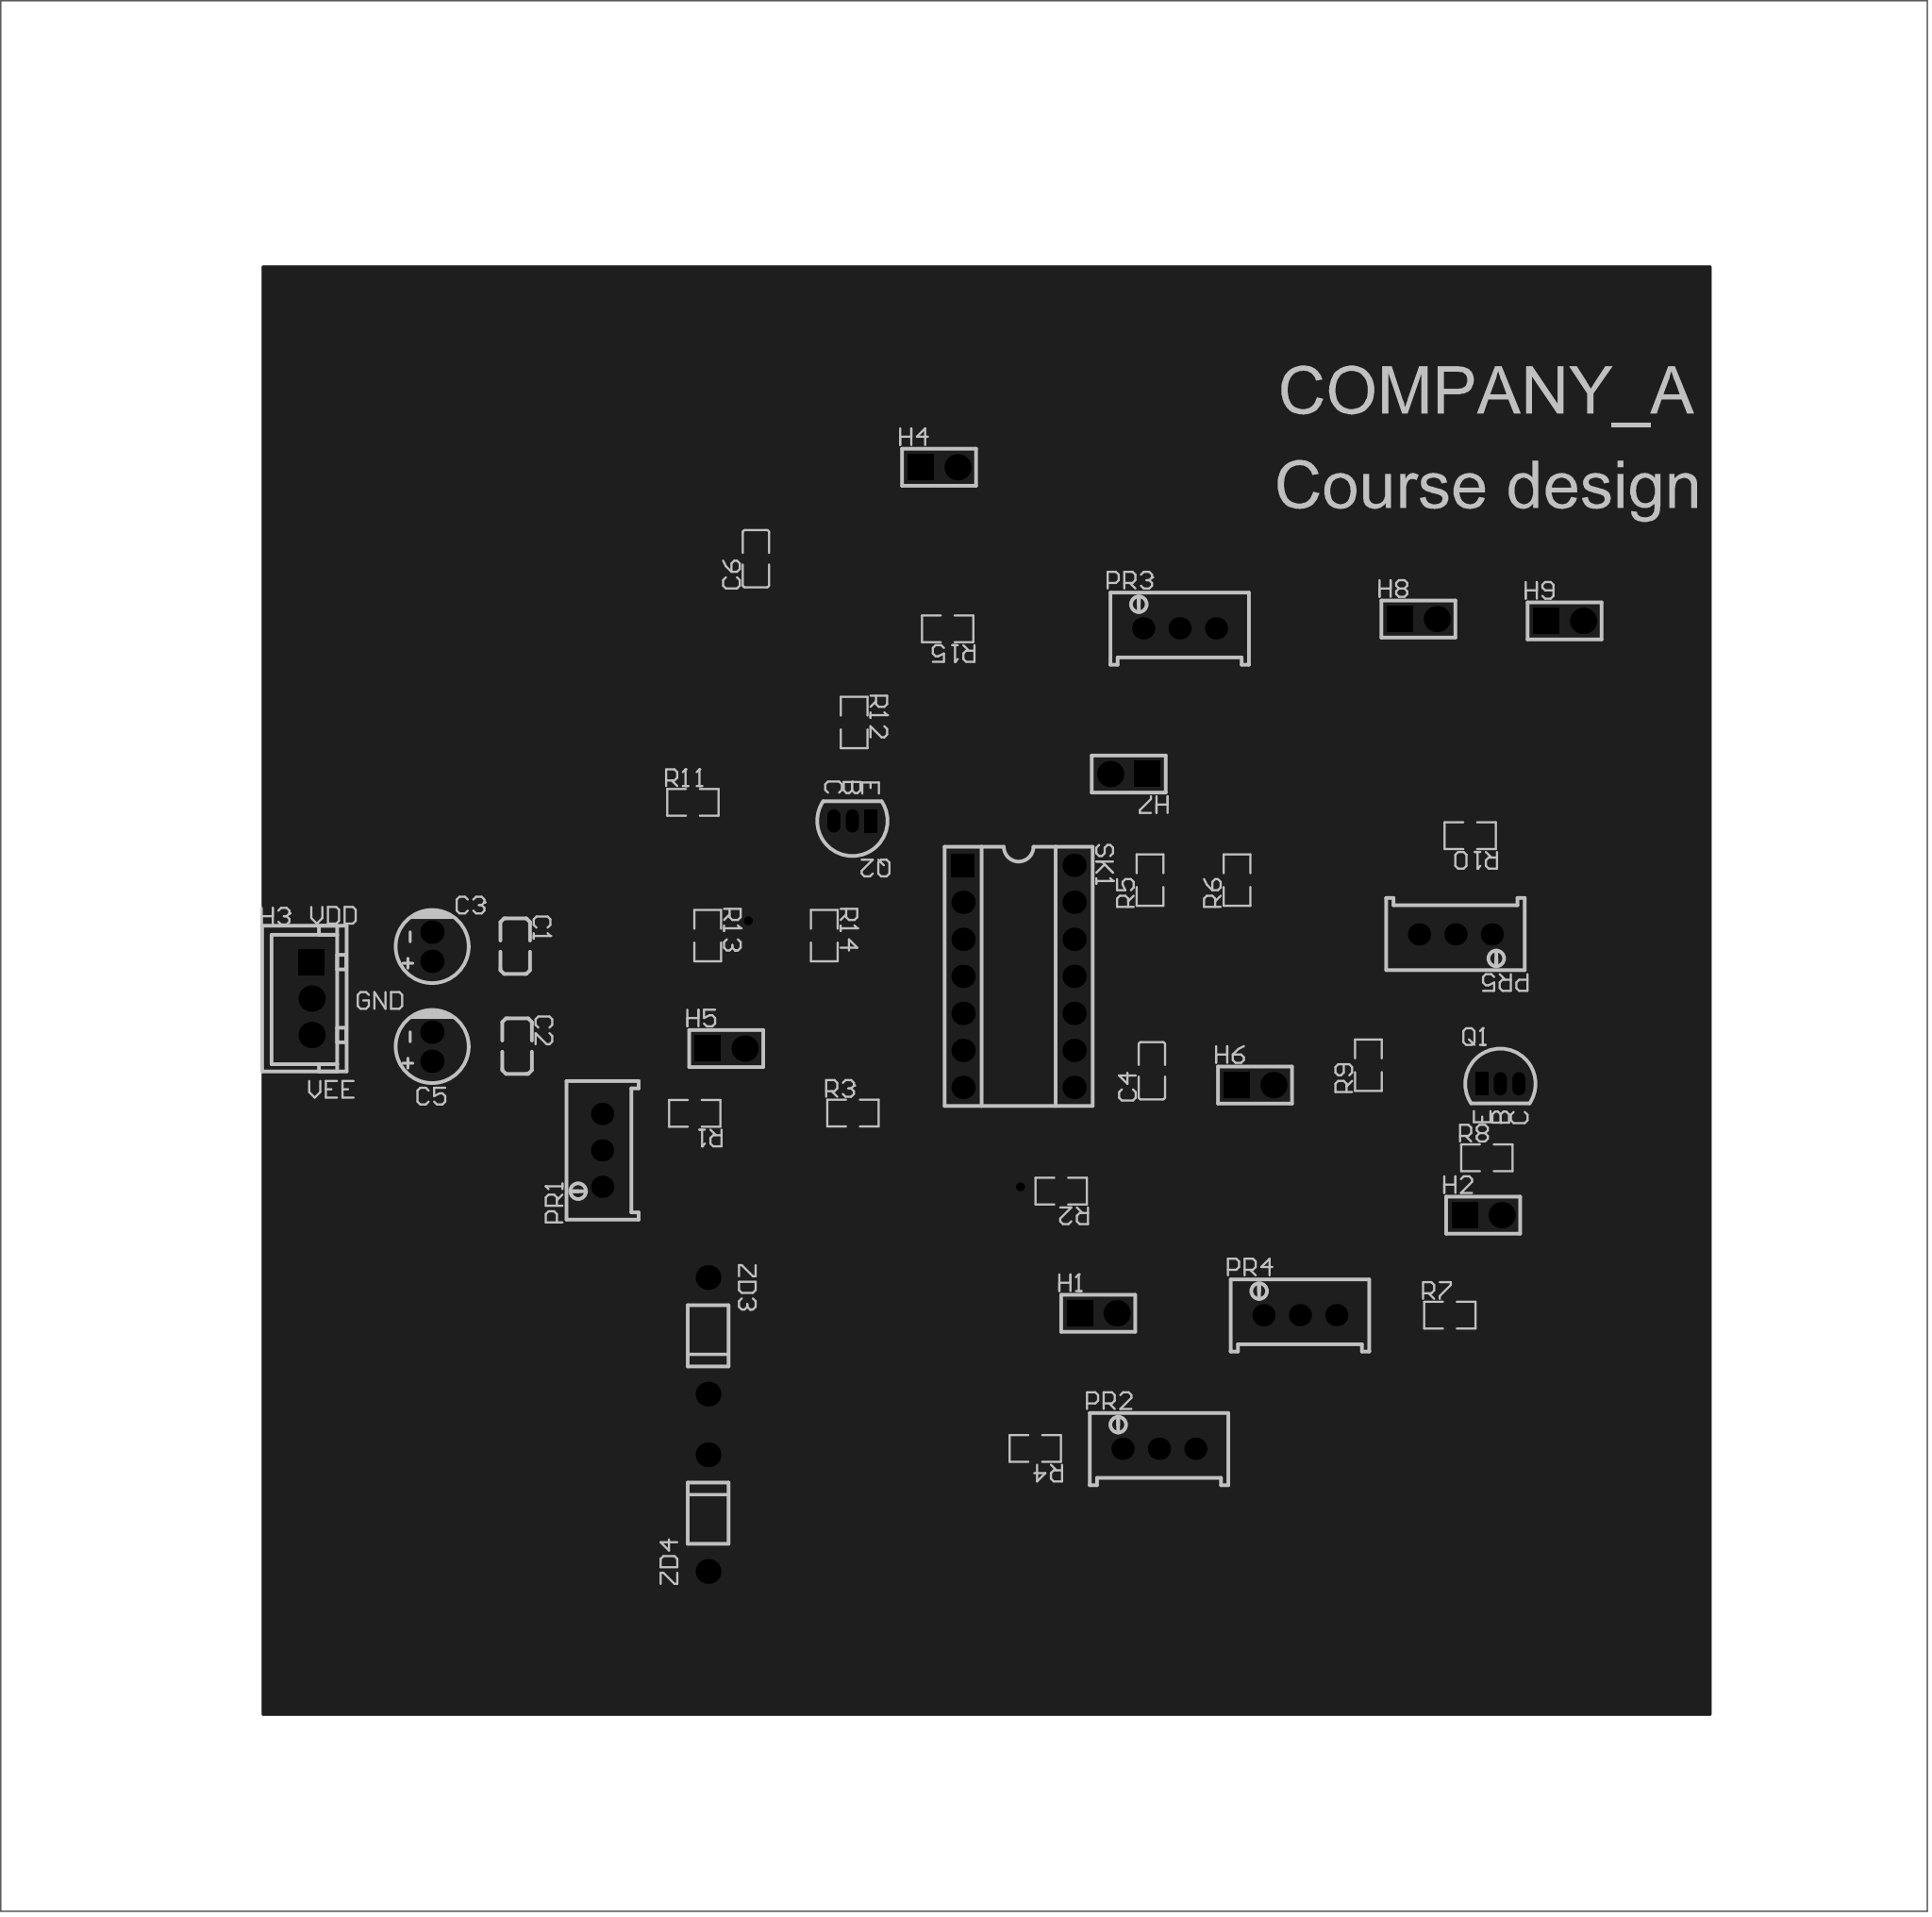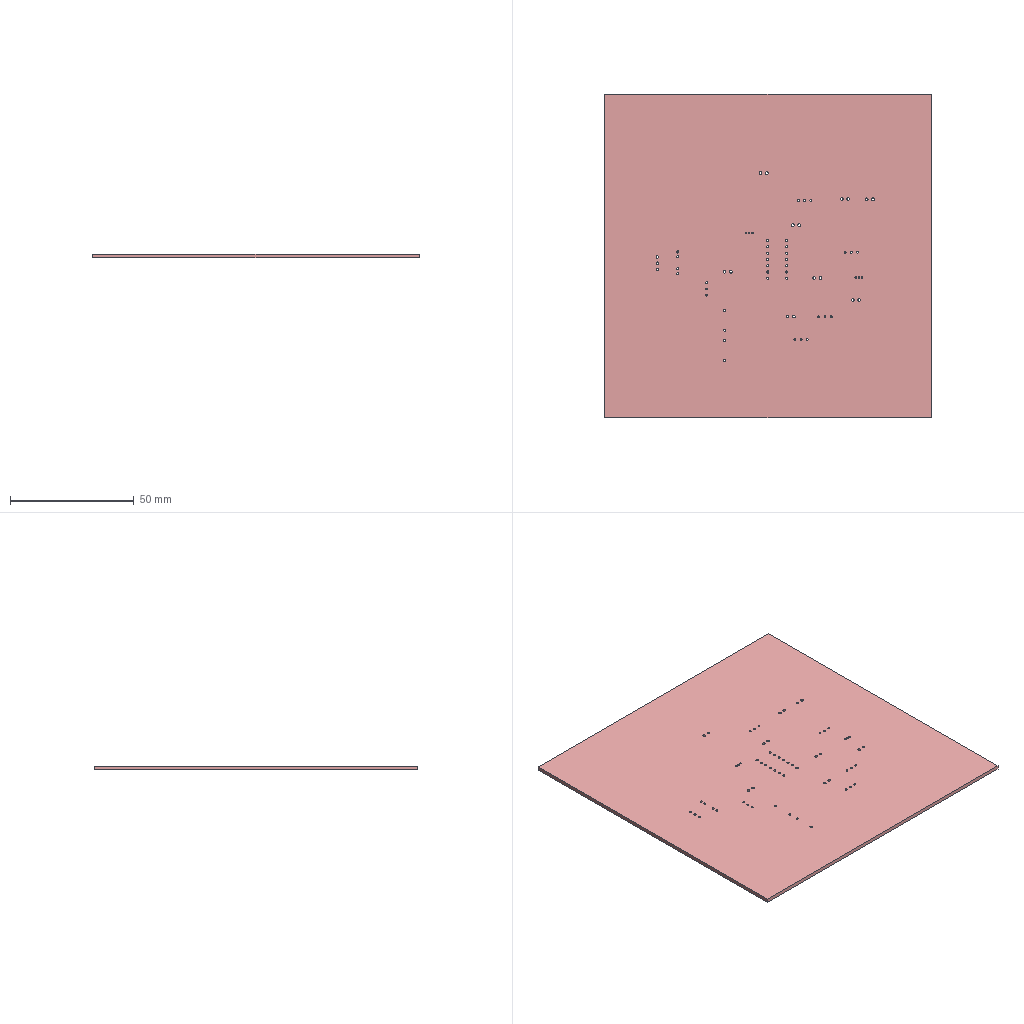Circuit board layout | Altium Designer | box 132.2 x 131.1 x 1.6 mm
Layer stack:
# Altium Designer layer stack of  (unit mm; dielectric type: 0 none, 1 core, 2 prepreg, 3 surface material)
index,name,kind,layer,copper_thickness_mm,dielectric_type,dielectric_thickness_mm,dielectric_material,dielectric_constant
0,Top Paste Mask Layer,other,,,,,,
1,Top Silkscreen Layer,other,,,,,,
2,Top Solder Mask Layer,dielectric,,,3,0.01,,3.3
3,Top Layer,copper,Top Layer,0.035,,,,
4,Dielectric1,dielectric,,,3,1.51,FR4,4.5
5,Bottom Layer,copper,Bottom Layer,0.035,,,,
6,Bottom Solder Mask Layer,dielectric,,,3,0.01,,3.3
7,Bottom Silkscreen Layer,other,,,,,,
8,Bottom Paste Mask Layer,other,,,,,,
# drill layer pairs: low layer,high layer
drill_pair,Top Layer,Bottom Layer
Part placement:
Designator,Comment,Layer,Footprint,Center-X(mm),Center-Y(mm),Rotation
C1,100nF,TopLayer,L0805,105.156,136.017,270
C2,100nF,TopLayer,L0805,105.283,129.159,270
C3,10uF,TopLayer,CAP-TH_BD5.0-P2.00-D0.5-FD-A,99.441,136.017,90
C4,22nF,TopLayer,C0805,148.844,127.508,90
C5,10uF,TopLayer,CAP-TH_BD5.0-P2.00-D0.5-FD-A,99.441,129.159,90
C6,100pF,TopLayer,C0805,121.671,162.635,90
H1,,TopLayer,HDR-TH_2P-P2.54-V-M-1,145.161,110.871,0
H2,,TopLayer,HDR-TH_2P-P2.54-V-M-1,171.577,117.602,0
H3,,TopLayer,CONN-TH_3P-P2.50_HX-XH2.54-3PZZ-B,91.186,132.461,90
H4,,TopLayer,HDR-TH_2P-P2.54-V-M-1,134.239,168.91,0
H5,,TopLayer,HDR-TH_2P-P2.54-V-M-1,119.634,129.032,0
H6,,TopLayer,HDR-TH_2P-P2.54-V-M-1,155.92,126.528,0
H7,,TopLayer,HDR-TH_2P-P2.54-V-M-1,147.256,147.864,180
H8,,TopLayer,HDR-TH_2P-P2.54-V-M-1,167.132,158.496,0
H9,,TopLayer,HDR-TH_2P-P2.54-V-M-1,177.165,158.369,0
PR1,5kΩ,TopLayer,R_3296,111.125,122.047,90
PR2,100kΩ,TopLayer,R_3296,149.333,101.578,0
PR3,10kΩ,TopLayer,R_3296,150.749,157.861,0
PR4,10kΩ,TopLayer,R_3296,159.004,110.744,0
PR5,10kΩ,TopLayer,R_3296,169.677,136.865,180
Q1,,TopLayer,S8050_TO_92,172.758,126.618,0
Q2,,TopLayer,S8050_TO_92,128.292,144.651,180
R1,20K,TopLayer,R0805,117.475,124.587,180
R2,20K,TopLayer,R0805,142.621,119.253,180
R3,1K,TopLayer,R0805,128.331,124.606,0
R4,4.7K,TopLayer,R0805,140.843,101.6,180
R5,12K,TopLayer,R0805,148.717,140.589,90
R6,10K,TopLayer,R0805,154.686,140.589,90
R7,2.2K,TopLayer,R0805,169.291,110.744,0
R8,220,TopLayer,R0805,171.831,121.539,0
R9,390,TopLayer,R0805,163.703,127.889,90
R10,10K,TopLayer,R0805,170.688,143.637,180
R11,4.7K,TopLayer,R0805,117.348,145.923,0
R12,220,TopLayer,R0805,128.413,151.4,270
R13,4.7K,TopLayer,R0805,118.364,136.779,270
R14,4.7K,TopLayer,R0805,126.365,136.779,270
R15,4.7K,TopLayer,R0805,134.831,157.825,180
SK1,LM324,TopLayer,DIP-14_L17.8-W10.2-P2.54-BL,139.7,133.985,270
ZD3,1N4733A,TopLayer,DO-41_BD2.8-L4.2-P8.00-D0.7-FD,118.393,109.325,270
ZD4,1N4733A,TopLayer,DO-41_BD2.8-L4.2-P8.00-D0.7-FD,118.393,97.16,90
Pad and via stacks:
# Altium Designer via and pad stacks of  (unit mm). Each distinct definition once, with the count of objects using it.
# via: kind,start_layer,end_layer,hole_mm,diameter_mm,mode(0 simple;1 top-mid-bottom;2 full stack),diameter_per_layer,count,example_net
# pad: kind,layer,hole_mm,hole_type(0 round;1 square;2 slot),plating,top_size,top_shape(1 round;2 rect;3 octagon;9 rounded rect),mid_size,bottom_size,mode,footprint,size_per_layer,count,example
pad,Top Layer,0,0,plated,1.133x1.377,2,1.133x1.377,1.133x1.377,0,L0805,,4,C1.1
pad,Top Layer,0,0,plated,1.41x1.35,2,1.41x1.35,1.41x1.35,0,C0805,,4,C4.2
pad,Top Layer,0,0,plated,1.133x1.377,2,1.133x1.377,1.133x1.377,0,R0805,,30,R1.2
pad,Top Layer,0,0,plated,0.6096x0.6096,1,0.6096x0.6096,0.6096x0.6096,0,,,23,TP1
pad,Multi-Layer,0.9,0,plated,1.6x1.6,1,1.6x1.6,1.6x1.6,0,CAP-TH_BD5.0-P2.00-D0.5-FD-A,,4,C3.2
pad,Multi-Layer,1.1,0,plated,1.8x1.8,1,1.8x1.8,1.8x1.8,0,HDR-TH_2P-P2.54-V-M-1,,8,H1.2
pad,Multi-Layer,1.1,0,plated,1.8x1.8,2,1.8x1.8,1.8x1.8,0,HDR-TH_2P-P2.54-V-M-1,,8,H1.1
pad,Multi-Layer,1,0,plated,1.8x1.8,1,1.8x1.8,1.8x1.8,0,CONN-TH_3P-P2.50_HX-XH2.54-3PZZ-B,,2,H3.3
pad,Multi-Layer,1,0,plated,1.8x1.8,2,1.8x1.8,1.8x1.8,0,CONN-TH_3P-P2.50_HX-XH2.54-3PZZ-B,,1,H3.1
pad,Multi-Layer,0.762,0,plated,1.524x1.524,1,1.524x1.524,1.524x1.524,0,R_3296,,15,PR1.2
pad,Multi-Layer,0.701,0,plated,0.8992x1.6,2,0.8992x1.6,0.8992x1.6,0,S8050_TO_92,,2,Q1.1
pad,Multi-Layer,0.701,0,plated,0.8992x1.6,1,0.8992x1.6,0.8992x1.6,0,S8050_TO_92,,4,Q1.2
pad,Multi-Layer,0.9,0,plated,1.6x1.6,2,1.6x1.6,1.6x1.6,0,DIP-14_L17.8-W10.2-P2.54-BL,,1,SK1.1
pad,Multi-Layer,0.9,0,plated,1.6x1.6,1,1.6x1.6,1.6x1.6,0,DIP-14_L17.8-W10.2-P2.54-BL,,13,SK1.2
pad,Multi-Layer,0.9,0,plated,1.7x1.7,1,1.7x1.7,1.7x1.7,0,DO-41_BD2.8-L4.2-P8.00-D0.7-FD,,4,ZD3.1
pad,Bottom Layer,0,0,plated,0.6096x0.6096,1,0.6096x0.6096,0.6096x0.6096,0,,,2,TP2
via,Top Layer,Bottom Layer,0.3048,0.61,0,,2,NET3
Copper pours:
name,layer,net,type(0 solid;1 hatched;2 none)
Top Layer-GND,Top Layer,GND,0
Bottom Layer-GND,Bottom Layer,GND,0